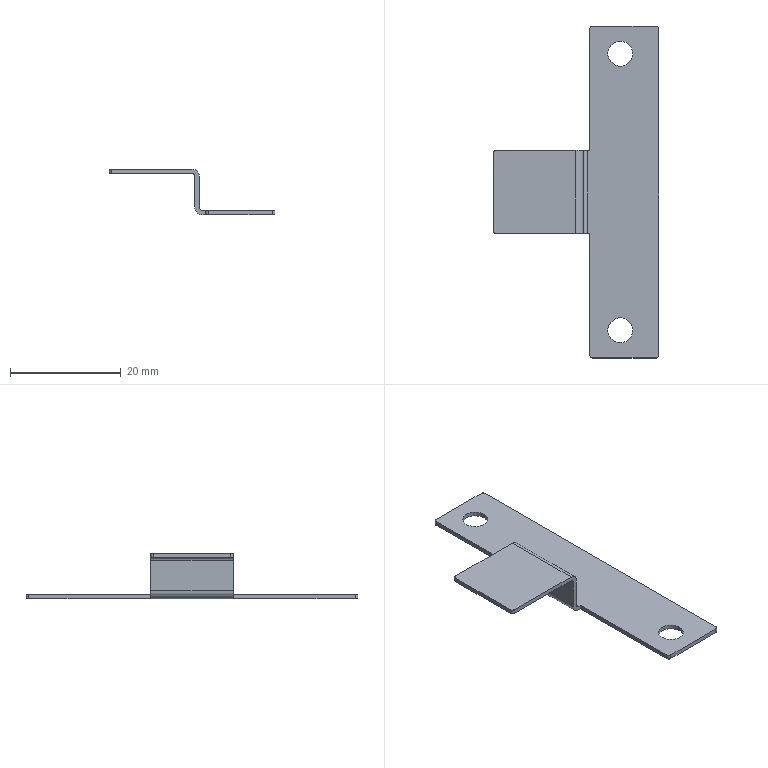Part | STEP file | 复件 FHB175-012^FHB175S-PRW-P40(马达RightUpper折-400W伺服电机) | 1 solid | 28 faces | box 30 x 60 x 8.3 mm | volume 863.995 mm3 | cylinder 14 | plane 14 | commonest cylinder face diameters 1 x7 4.5 x4 1.4 x1 2.6 x1 3 x1
STEP:
#1=CARTESIAN_POINT('',(7.253,-3.586,0.));
#2=VERTEX_POINT('',#1);
#3=CARTESIAN_POINT('',(11.753,-3.586,0.));
#4=VERTEX_POINT('',#3);
#5=CARTESIAN_POINT('',(9.503,-3.586,0.));
#6=DIRECTION('',(0.,0.,1.));
#7=DIRECTION('',(1.,0.,0.));
#8=AXIS2_PLACEMENT_3D('',#5,#6,#7);
#9=CIRCLE('',#8,2.25);
#10=EDGE_CURVE('',#2,#4,#9,.T.);
#11=ORIENTED_EDGE('',*,*,#10,.F.);
#12=CARTESIAN_POINT('',(7.253,-3.586,0.8));
#13=VERTEX_POINT('',#12);
#14=CARTESIAN_POINT('',(7.253,-3.586,0.8));
#15=DIRECTION('',(0.,0.,1.));
#16=VECTOR('',#15,1000.);
#17=LINE('',#14,#16);
#18=EDGE_CURVE('',#2,#13,#17,.T.);
#19=ORIENTED_EDGE('',*,*,#18,.T.);
#20=CARTESIAN_POINT('',(11.753,-3.586,0.8));
#21=VERTEX_POINT('',#20);
#22=CARTESIAN_POINT('',(9.503,-3.586,0.8));
#23=DIRECTION('',(0.,0.,-1.));
#24=DIRECTION('',(1.,0.,0.));
#25=AXIS2_PLACEMENT_3D('',#22,#23,#24);
#26=CIRCLE('',#25,2.25);
#27=EDGE_CURVE('',#21,#13,#26,.T.);
#28=ORIENTED_EDGE('',*,*,#27,.F.);
#29=CARTESIAN_POINT('',(11.753,-3.586,0.8));
#30=DIRECTION('',(0.,0.,1.));
#31=VECTOR('',#30,1000.);
#32=LINE('',#29,#31);
#33=EDGE_CURVE('',#4,#21,#32,.T.);
#34=ORIENTED_EDGE('',*,*,#33,.F.);
#35=EDGE_LOOP('',(#11,#19,#28,#34));
#36=FACE_OUTER_BOUND('',#35,.T.);
#37=CARTESIAN_POINT('',(9.503,-3.586,0.8));
#38=DIRECTION('',(0.,0.,1.));
#39=DIRECTION('',(1.,0.,0.));
#40=AXIS2_PLACEMENT_3D('',#37,#38,#39);
#41=CYLINDRICAL_SURFACE('',#40,2.25);
#42=ADVANCED_FACE('',(#36),#41,.F.);
#43=CARTESIAN_POINT('',(7.253,46.414,0.));
#44=VERTEX_POINT('',#43);
#45=CARTESIAN_POINT('',(11.753,46.414,0.));
#46=VERTEX_POINT('',#45);
#47=CARTESIAN_POINT('',(9.503,46.414,0.));
#48=DIRECTION('',(0.,0.,1.));
#49=DIRECTION('',(1.,0.,0.));
#50=AXIS2_PLACEMENT_3D('',#47,#48,#49);
#51=CIRCLE('',#50,2.25);
#52=EDGE_CURVE('',#44,#46,#51,.T.);
#53=ORIENTED_EDGE('',*,*,#52,.F.);
#54=CARTESIAN_POINT('',(7.253,46.414,0.8));
#55=VERTEX_POINT('',#54);
#56=CARTESIAN_POINT('',(7.253,46.414,0.8));
#57=DIRECTION('',(0.,0.,1.));
#58=VECTOR('',#57,1000.);
#59=LINE('',#56,#58);
#60=EDGE_CURVE('',#44,#55,#59,.T.);
#61=ORIENTED_EDGE('',*,*,#60,.T.);
#62=CARTESIAN_POINT('',(11.753,46.414,0.8));
#63=VERTEX_POINT('',#62);
#64=CARTESIAN_POINT('',(9.503,46.414,0.8));
#65=DIRECTION('',(0.,0.,-1.));
#66=DIRECTION('',(1.,0.,0.));
#67=AXIS2_PLACEMENT_3D('',#64,#65,#66);
#68=CIRCLE('',#67,2.25);
#69=EDGE_CURVE('',#63,#55,#68,.T.);
#70=ORIENTED_EDGE('',*,*,#69,.F.);
#71=CARTESIAN_POINT('',(11.753,46.414,0.8));
#72=DIRECTION('',(0.,0.,1.));
#73=VECTOR('',#72,1000.);
#74=LINE('',#71,#73);
#75=EDGE_CURVE('',#46,#63,#74,.T.);
#76=ORIENTED_EDGE('',*,*,#75,.F.);
#77=EDGE_LOOP('',(#53,#61,#70,#76));
#78=FACE_OUTER_BOUND('',#77,.T.);
#79=CARTESIAN_POINT('',(9.503,46.414,0.8));
#80=DIRECTION('',(0.,0.,1.));
#81=DIRECTION('',(1.,0.,0.));
#82=AXIS2_PLACEMENT_3D('',#79,#80,#81);
#83=CYLINDRICAL_SURFACE('',#82,2.25);
#84=ADVANCED_FACE('',(#78),#83,.F.);
#85=CARTESIAN_POINT('',(16.503,50.914,0.));
#86=VERTEX_POINT('',#85);
#87=CARTESIAN_POINT('',(16.503,-8.086,0.));
#88=VERTEX_POINT('',#87);
#89=CARTESIAN_POINT('',(16.503,0.,0.));
#90=DIRECTION('',(0.,-1.,0.));
#91=VECTOR('',#90,1000.);
#92=LINE('',#89,#91);
#93=EDGE_CURVE('',#86,#88,#92,.T.);
#94=ORIENTED_EDGE('',*,*,#93,.T.);
#95=CARTESIAN_POINT('',(16.003,-8.586,0.));
#96=VERTEX_POINT('',#95);
#97=CARTESIAN_POINT('',(16.003,-8.086,0.));
#98=DIRECTION('',(0.,0.,-1.));
#99=DIRECTION('',(-1.,0.,0.));
#100=AXIS2_PLACEMENT_3D('',#97,#98,#99);
#101=CIRCLE('',#100,0.5);
#102=EDGE_CURVE('',#88,#96,#101,.T.);
#103=ORIENTED_EDGE('',*,*,#102,.T.);
#104=CARTESIAN_POINT('',(4.503,-8.586,0.));
#105=VERTEX_POINT('',#104);
#106=CARTESIAN_POINT('',(0.,-8.586,0.));
#107=DIRECTION('',(-1.,0.,0.));
#108=VECTOR('',#107,1000.);
#109=LINE('',#106,#108);
#110=EDGE_CURVE('',#96,#105,#109,.T.);
#111=ORIENTED_EDGE('',*,*,#110,.T.);
#112=CARTESIAN_POINT('',(4.003,-8.086,0.));
#113=VERTEX_POINT('',#112);
#114=CARTESIAN_POINT('',(4.503,-8.086,0.));
#115=DIRECTION('',(0.,0.,-1.));
#116=DIRECTION('',(1.,0.,0.));
#117=AXIS2_PLACEMENT_3D('',#114,#115,#116);
#118=CIRCLE('',#117,0.5);
#119=EDGE_CURVE('',#105,#113,#118,.T.);
#120=ORIENTED_EDGE('',*,*,#119,.T.);
#121=CARTESIAN_POINT('',(4.003,13.914,0.));
#122=VERTEX_POINT('',#121);
#123=CARTESIAN_POINT('',(4.003,0.,0.));
#124=DIRECTION('',(0.,1.,0.));
#125=VECTOR('',#124,1000.);
#126=LINE('',#123,#125);
#127=EDGE_CURVE('',#113,#122,#126,.T.);
#128=ORIENTED_EDGE('',*,*,#127,.T.);
#129=CARTESIAN_POINT('',(3.503,13.914,0.));
#130=VERTEX_POINT('',#129);
#131=CARTESIAN_POINT('',(0.,13.914,0.));
#132=DIRECTION('',(-1.,0.,0.));
#133=VECTOR('',#132,1000.);
#134=LINE('',#131,#133);
#135=EDGE_CURVE('',#122,#130,#134,.T.);
#136=ORIENTED_EDGE('',*,*,#135,.T.);
#137=CARTESIAN_POINT('',(3.503,28.914,0.));
#138=VERTEX_POINT('',#137);
#139=CARTESIAN_POINT('',(3.503,0.,0.));
#140=DIRECTION('',(0.,1.,0.));
#141=VECTOR('',#140,1000.);
#142=LINE('',#139,#141);
#143=EDGE_CURVE('',#130,#138,#142,.T.);
#144=ORIENTED_EDGE('',*,*,#143,.T.);
#145=CARTESIAN_POINT('',(4.003,28.914,0.));
#146=VERTEX_POINT('',#145);
#147=CARTESIAN_POINT('',(0.,28.914,0.));
#148=DIRECTION('',(1.,0.,0.));
#149=VECTOR('',#148,1000.);
#150=LINE('',#147,#149);
#151=EDGE_CURVE('',#138,#146,#150,.T.);
#152=ORIENTED_EDGE('',*,*,#151,.T.);
#153=CARTESIAN_POINT('',(4.003,50.914,0.));
#154=VERTEX_POINT('',#153);
#155=CARTESIAN_POINT('',(4.003,0.,0.));
#156=DIRECTION('',(0.,1.,0.));
#157=VECTOR('',#156,1000.);
#158=LINE('',#155,#157);
#159=EDGE_CURVE('',#146,#154,#158,.T.);
#160=ORIENTED_EDGE('',*,*,#159,.T.);
#161=CARTESIAN_POINT('',(4.503,51.414,0.));
#162=VERTEX_POINT('',#161);
#163=CARTESIAN_POINT('',(4.503,50.914,0.));
#164=DIRECTION('',(0.,0.,-1.));
#165=DIRECTION('',(1.,0.,0.));
#166=AXIS2_PLACEMENT_3D('',#163,#164,#165);
#167=CIRCLE('',#166,0.5);
#168=EDGE_CURVE('',#154,#162,#167,.T.);
#169=ORIENTED_EDGE('',*,*,#168,.T.);
#170=CARTESIAN_POINT('',(16.003,51.414,0.));
#171=VERTEX_POINT('',#170);
#172=CARTESIAN_POINT('',(0.,51.414,0.));
#173=DIRECTION('',(1.,0.,0.));
#174=VECTOR('',#173,1000.);
#175=LINE('',#172,#174);
#176=EDGE_CURVE('',#162,#171,#175,.T.);
#177=ORIENTED_EDGE('',*,*,#176,.T.);
#178=CARTESIAN_POINT('',(16.003,50.914,0.));
#179=DIRECTION('',(0.,0.,-1.));
#180=DIRECTION('',(-1.,0.,0.));
#181=AXIS2_PLACEMENT_3D('',#178,#179,#180);
#182=CIRCLE('',#181,0.5);
#183=EDGE_CURVE('',#171,#86,#182,.T.);
#184=ORIENTED_EDGE('',*,*,#183,.T.);
#185=EDGE_LOOP('',(#94,#103,#111,#120,#128,#136,#144,#152,#160,#169,#177,#184));
#186=FACE_OUTER_BOUND('',#185,.T.);
#187=CARTESIAN_POINT('',(9.503,-3.586,0.));
#188=DIRECTION('',(0.,0.,1.));
#189=DIRECTION('',(1.,0.,0.));
#190=AXIS2_PLACEMENT_3D('',#187,#188,#189);
#191=CIRCLE('',#190,2.25);
#192=EDGE_CURVE('',#4,#2,#191,.T.);
#193=ORIENTED_EDGE('',*,*,#192,.T.);
#194=ORIENTED_EDGE('',*,*,#10,.T.);
#195=EDGE_LOOP('',(#193,#194));
#196=FACE_BOUND('',#195,.T.);
#197=CARTESIAN_POINT('',(9.503,46.414,0.));
#198=DIRECTION('',(0.,0.,1.));
#199=DIRECTION('',(1.,0.,0.));
#200=AXIS2_PLACEMENT_3D('',#197,#198,#199);
#201=CIRCLE('',#200,2.25);
#202=EDGE_CURVE('',#46,#44,#201,.T.);
#203=ORIENTED_EDGE('',*,*,#202,.T.);
#204=ORIENTED_EDGE('',*,*,#52,.T.);
#205=EDGE_LOOP('',(#203,#204));
#206=FACE_BOUND('',#205,.T.);
#207=CARTESIAN_POINT('',(0.,0.,0.));
#208=DIRECTION('',(0.,0.,-1.));
#209=DIRECTION('',(-1.,0.,0.));
#210=AXIS2_PLACEMENT_3D('',#207,#208,#209);
#211=PLANE('',#210);
#212=ADVANCED_FACE('',(#186,#196,#206),#211,.T.);
#213=ORIENTED_EDGE('',*,*,#102,.F.);
#214=CARTESIAN_POINT('',(16.503,-8.086,0.8));
#215=VERTEX_POINT('',#214);
#216=CARTESIAN_POINT('',(16.503,-8.086,0.8));
#217=DIRECTION('',(0.,0.,1.));
#218=VECTOR('',#217,1000.);
#219=LINE('',#216,#218);
#220=EDGE_CURVE('',#88,#215,#219,.T.);
#221=ORIENTED_EDGE('',*,*,#220,.T.);
#222=CARTESIAN_POINT('',(16.003,-8.586,0.8));
#223=VERTEX_POINT('',#222);
#224=CARTESIAN_POINT('',(16.003,-8.086,0.8));
#225=DIRECTION('',(0.,0.,-1.));
#226=DIRECTION('',(-1.,0.,0.));
#227=AXIS2_PLACEMENT_3D('',#224,#225,#226);
#228=CIRCLE('',#227,0.5);
#229=EDGE_CURVE('',#215,#223,#228,.T.);
#230=ORIENTED_EDGE('',*,*,#229,.T.);
#231=CARTESIAN_POINT('',(16.003,-8.586,0.8));
#232=DIRECTION('',(0.,0.,-1.));
#233=VECTOR('',#232,1000.);
#234=LINE('',#231,#233);
#235=EDGE_CURVE('',#223,#96,#234,.T.);
#236=ORIENTED_EDGE('',*,*,#235,.T.);
#237=EDGE_LOOP('',(#213,#221,#230,#236));
#238=FACE_OUTER_BOUND('',#237,.T.);
#239=CARTESIAN_POINT('',(16.003,-8.086,0.8));
#240=DIRECTION('',(0.,0.,-1.));
#241=DIRECTION('',(-1.,0.,0.));
#242=AXIS2_PLACEMENT_3D('',#239,#240,#241);
#243=CYLINDRICAL_SURFACE('',#242,0.5);
#244=ADVANCED_FACE('',(#238),#243,.T.);
#245=ORIENTED_EDGE('',*,*,#220,.F.);
#246=ORIENTED_EDGE('',*,*,#93,.F.);
#247=CARTESIAN_POINT('',(16.503,50.914,0.8));
#248=VERTEX_POINT('',#247);
#249=CARTESIAN_POINT('',(16.503,50.914,0.8));
#250=DIRECTION('',(0.,0.,-1.));
#251=VECTOR('',#250,1000.);
#252=LINE('',#249,#251);
#253=EDGE_CURVE('',#248,#86,#252,.T.);
#254=ORIENTED_EDGE('',*,*,#253,.F.);
#255=CARTESIAN_POINT('',(16.503,51.414,0.8));
#256=DIRECTION('',(0.,1.,0.));
#257=VECTOR('',#256,1000.);
#258=LINE('',#255,#257);
#259=EDGE_CURVE('',#215,#248,#258,.T.);
#260=ORIENTED_EDGE('',*,*,#259,.F.);
#261=EDGE_LOOP('',(#245,#246,#254,#260));
#262=FACE_OUTER_BOUND('',#261,.T.);
#263=CARTESIAN_POINT('',(16.503,51.414,0.8));
#264=DIRECTION('',(-1.,0.,0.));
#265=DIRECTION('',(0.,-1.,0.));
#266=AXIS2_PLACEMENT_3D('',#263,#264,#265);
#267=PLANE('',#266);
#268=ADVANCED_FACE('',(#262),#267,.F.);
#269=ORIENTED_EDGE('',*,*,#183,.F.);
#270=CARTESIAN_POINT('',(16.003,51.414,0.8));
#271=VERTEX_POINT('',#270);
#272=CARTESIAN_POINT('',(16.003,51.414,0.8));
#273=DIRECTION('',(0.,0.,1.));
#274=VECTOR('',#273,1000.);
#275=LINE('',#272,#274);
#276=EDGE_CURVE('',#171,#271,#275,.T.);
#277=ORIENTED_EDGE('',*,*,#276,.T.);
#278=CARTESIAN_POINT('',(16.003,50.914,0.8));
#279=DIRECTION('',(0.,0.,-1.));
#280=DIRECTION('',(-1.,0.,0.));
#281=AXIS2_PLACEMENT_3D('',#278,#279,#280);
#282=CIRCLE('',#281,0.5);
#283=EDGE_CURVE('',#271,#248,#282,.T.);
#284=ORIENTED_EDGE('',*,*,#283,.T.);
#285=ORIENTED_EDGE('',*,*,#253,.T.);
#286=EDGE_LOOP('',(#269,#277,#284,#285));
#287=FACE_OUTER_BOUND('',#286,.T.);
#288=CARTESIAN_POINT('',(16.003,50.914,0.8));
#289=DIRECTION('',(0.,0.,-1.));
#290=DIRECTION('',(-1.,0.,0.));
#291=AXIS2_PLACEMENT_3D('',#288,#289,#290);
#292=CYLINDRICAL_SURFACE('',#291,0.5);
#293=ADVANCED_FACE('',(#287),#292,.T.);
#294=CARTESIAN_POINT('',(4.503,51.414,0.8));
#295=VERTEX_POINT('',#294);
#296=CARTESIAN_POINT('',(4.503,51.414,0.8));
#297=DIRECTION('',(0.,0.,-1.));
#298=VECTOR('',#297,1000.);
#299=LINE('',#296,#298);
#300=EDGE_CURVE('',#295,#162,#299,.T.);
#301=ORIENTED_EDGE('',*,*,#300,.F.);
#302=CARTESIAN_POINT('',(16.503,51.414,0.8));
#303=DIRECTION('',(-1.,0.,0.));
#304=VECTOR('',#303,1000.);
#305=LINE('',#302,#304);
#306=EDGE_CURVE('',#271,#295,#305,.T.);
#307=ORIENTED_EDGE('',*,*,#306,.F.);
#308=ORIENTED_EDGE('',*,*,#276,.F.);
#309=ORIENTED_EDGE('',*,*,#176,.F.);
#310=EDGE_LOOP('',(#301,#307,#308,#309));
#311=FACE_OUTER_BOUND('',#310,.T.);
#312=CARTESIAN_POINT('',(16.503,51.414,0.8));
#313=DIRECTION('',(0.,-1.,0.));
#314=DIRECTION('',(0.,0.,-1.));
#315=AXIS2_PLACEMENT_3D('',#312,#313,#314);
#316=PLANE('',#315);
#317=ADVANCED_FACE('',(#311),#316,.F.);
#318=CARTESIAN_POINT('',(4.003,50.914,0.8));
#319=VERTEX_POINT('',#318);
#320=CARTESIAN_POINT('',(4.503,50.914,0.8));
#321=DIRECTION('',(0.,0.,-1.));
#322=DIRECTION('',(1.,0.,0.));
#323=AXIS2_PLACEMENT_3D('',#320,#321,#322);
#324=CIRCLE('',#323,0.5);
#325=EDGE_CURVE('',#319,#295,#324,.T.);
#326=ORIENTED_EDGE('',*,*,#325,.T.);
#327=ORIENTED_EDGE('',*,*,#300,.T.);
#328=ORIENTED_EDGE('',*,*,#168,.F.);
#329=CARTESIAN_POINT('',(4.003,50.914,0.8));
#330=DIRECTION('',(0.,0.,1.));
#331=VECTOR('',#330,1000.);
#332=LINE('',#329,#331);
#333=EDGE_CURVE('',#154,#319,#332,.T.);
#334=ORIENTED_EDGE('',*,*,#333,.T.);
#335=EDGE_LOOP('',(#326,#327,#328,#334));
#336=FACE_OUTER_BOUND('',#335,.T.);
#337=CARTESIAN_POINT('',(4.503,50.914,0.8));
#338=DIRECTION('',(0.,0.,1.));
#339=DIRECTION('',(1.,0.,0.));
#340=AXIS2_PLACEMENT_3D('',#337,#338,#339);
#341=CYLINDRICAL_SURFACE('',#340,0.5);
#342=ADVANCED_FACE('',(#336),#341,.T.);
#343=ORIENTED_EDGE('',*,*,#333,.F.);
#344=ORIENTED_EDGE('',*,*,#159,.F.);
#345=CARTESIAN_POINT('',(4.003,28.914,0.8));
#346=VERTEX_POINT('',#345);
#347=CARTESIAN_POINT('',(4.003,28.914,0.));
#348=DIRECTION('',(0.,0.,-1.));
#349=VECTOR('',#348,1000.);
#350=LINE('',#347,#349);
#351=EDGE_CURVE('',#346,#146,#350,.T.);
#352=ORIENTED_EDGE('',*,*,#351,.F.);
#353=CARTESIAN_POINT('',(4.003,51.414,0.8));
#354=DIRECTION('',(0.,-1.,0.));
#355=VECTOR('',#354,1000.);
#356=LINE('',#353,#355);
#357=EDGE_CURVE('',#319,#346,#356,.T.);
#358=ORIENTED_EDGE('',*,*,#357,.F.);
#359=EDGE_LOOP('',(#343,#344,#352,#358));
#360=FACE_OUTER_BOUND('',#359,.T.);
#361=CARTESIAN_POINT('',(4.003,51.414,0.));
#362=DIRECTION('',(1.,0.,0.));
#363=DIRECTION('',(0.,1.,0.));
#364=AXIS2_PLACEMENT_3D('',#361,#362,#363);
#365=PLANE('',#364);
#366=ADVANCED_FACE('',(#360),#365,.F.);
#367=ORIENTED_EDGE('',*,*,#351,.T.);
#368=ORIENTED_EDGE('',*,*,#151,.F.);
#369=CARTESIAN_POINT('',(2.003,28.914,1.5));
#370=VERTEX_POINT('',#369);
#371=CARTESIAN_POINT('',(3.503,28.914,1.5));
#372=DIRECTION('',(0.,-1.,0.));
#373=DIRECTION('',(0.,0.,-1.));
#374=AXIS2_PLACEMENT_3D('',#371,#372,#373);
#375=CIRCLE('',#374,1.5);
#376=EDGE_CURVE('',#370,#138,#375,.T.);
#377=ORIENTED_EDGE('',*,*,#376,.F.);
#378=CARTESIAN_POINT('',(2.003,28.914,7.));
#379=VERTEX_POINT('',#378);
#380=CARTESIAN_POINT('',(2.003,28.914,0.));
#381=DIRECTION('',(0.,0.,1.));
#382=VECTOR('',#381,1000.);
#383=LINE('',#380,#382);
#384=EDGE_CURVE('',#370,#379,#383,.T.);
#385=ORIENTED_EDGE('',*,*,#384,.T.);
#386=CARTESIAN_POINT('',(1.503,28.914,7.5));
#387=VERTEX_POINT('',#386);
#388=CARTESIAN_POINT('',(1.503,28.914,7.));
#389=DIRECTION('',(0.,1.,0.));
#390=DIRECTION('',(0.,0.,1.));
#391=AXIS2_PLACEMENT_3D('',#388,#389,#390);
#392=CIRCLE('',#391,0.5);
#393=EDGE_CURVE('',#387,#379,#392,.T.);
#394=ORIENTED_EDGE('',*,*,#393,.F.);
#395=CARTESIAN_POINT('',(-12.997,28.914,7.5));
#396=VERTEX_POINT('',#395);
#397=CARTESIAN_POINT('',(0.,28.914,7.5));
#398=DIRECTION('',(-1.,0.,0.));
#399=VECTOR('',#398,1000.);
#400=LINE('',#397,#399);
#401=EDGE_CURVE('',#387,#396,#400,.T.);
#402=ORIENTED_EDGE('',*,*,#401,.T.);
#403=CARTESIAN_POINT('',(-12.997,28.914,8.3));
#404=VERTEX_POINT('',#403);
#405=CARTESIAN_POINT('',(-12.997,28.914,8.3));
#406=DIRECTION('',(0.,0.,-1.));
#407=VECTOR('',#406,1000.);
#408=LINE('',#405,#407);
#409=EDGE_CURVE('',#404,#396,#408,.T.);
#410=ORIENTED_EDGE('',*,*,#409,.F.);
#411=CARTESIAN_POINT('',(1.503,28.914,8.3));
#412=VERTEX_POINT('',#411);
#413=CARTESIAN_POINT('',(2.003,28.914,8.3));
#414=DIRECTION('',(1.,0.,0.));
#415=VECTOR('',#414,1000.);
#416=LINE('',#413,#415);
#417=EDGE_CURVE('',#404,#412,#416,.T.);
#418=ORIENTED_EDGE('',*,*,#417,.T.);
#419=CARTESIAN_POINT('',(2.803,28.914,7.));
#420=VERTEX_POINT('',#419);
#421=CARTESIAN_POINT('',(1.503,28.914,7.));
#422=DIRECTION('',(0.,-1.,0.));
#423=DIRECTION('',(0.,0.,1.));
#424=AXIS2_PLACEMENT_3D('',#421,#422,#423);
#425=CIRCLE('',#424,1.3);
#426=EDGE_CURVE('',#420,#412,#425,.T.);
#427=ORIENTED_EDGE('',*,*,#426,.F.);
#428=CARTESIAN_POINT('',(2.803,28.914,1.5));
#429=VERTEX_POINT('',#428);
#430=CARTESIAN_POINT('',(2.803,28.914,0.8));
#431=DIRECTION('',(0.,0.,1.));
#432=VECTOR('',#431,1000.);
#433=LINE('',#430,#432);
#434=EDGE_CURVE('',#429,#420,#433,.T.);
#435=ORIENTED_EDGE('',*,*,#434,.F.);
#436=CARTESIAN_POINT('',(3.503,28.914,0.8));
#437=VERTEX_POINT('',#436);
#438=CARTESIAN_POINT('',(3.503,28.914,1.5));
#439=DIRECTION('',(0.,-1.,0.));
#440=DIRECTION('',(0.,0.,-1.));
#441=AXIS2_PLACEMENT_3D('',#438,#439,#440);
#442=CIRCLE('',#441,0.7);
#443=EDGE_CURVE('',#429,#437,#442,.T.);
#444=ORIENTED_EDGE('',*,*,#443,.T.);
#445=CARTESIAN_POINT('',(4.003,28.914,0.8));
#446=DIRECTION('',(-1.,0.,0.));
#447=VECTOR('',#446,1000.);
#448=LINE('',#445,#447);
#449=EDGE_CURVE('',#346,#437,#448,.T.);
#450=ORIENTED_EDGE('',*,*,#449,.F.);
#451=EDGE_LOOP('',(#367,#368,#377,#385,#394,#402,#410,#418,#427,#435,#444,#450));
#452=FACE_OUTER_BOUND('',#451,.T.);
#453=CARTESIAN_POINT('',(4.003,28.914,0.));
#454=DIRECTION('',(0.,-1.,0.));
#455=DIRECTION('',(0.,0.,-1.));
#456=AXIS2_PLACEMENT_3D('',#453,#454,#455);
#457=PLANE('',#456);
#458=ADVANCED_FACE('',(#452),#457,.F.);
#459=CARTESIAN_POINT('',(2.003,13.914,1.5));
#460=VERTEX_POINT('',#459);
#461=CARTESIAN_POINT('',(2.003,13.914,1.5));
#462=DIRECTION('',(0.,1.,0.));
#463=VECTOR('',#462,1000.);
#464=LINE('',#461,#463);
#465=EDGE_CURVE('',#460,#370,#464,.T.);
#466=ORIENTED_EDGE('',*,*,#465,.T.);
#467=ORIENTED_EDGE('',*,*,#376,.T.);
#468=ORIENTED_EDGE('',*,*,#143,.F.);
#469=CARTESIAN_POINT('',(3.503,13.914,1.5));
#470=DIRECTION('',(0.,1.,0.));
#471=DIRECTION('',(0.,0.,-1.));
#472=AXIS2_PLACEMENT_3D('',#469,#470,#471);
#473=CIRCLE('',#472,1.5);
#474=EDGE_CURVE('',#130,#460,#473,.T.);
#475=ORIENTED_EDGE('',*,*,#474,.T.);
#476=EDGE_LOOP('',(#466,#467,#468,#475));
#477=FACE_OUTER_BOUND('',#476,.T.);
#478=CARTESIAN_POINT('',(3.503,13.914,1.5));
#479=DIRECTION('',(0.,-1.,0.));
#480=DIRECTION('',(0.,0.,-1.));
#481=AXIS2_PLACEMENT_3D('',#478,#479,#480);
#482=CYLINDRICAL_SURFACE('',#481,1.5);
#483=ADVANCED_FACE('',(#477),#482,.T.);
#484=CARTESIAN_POINT('',(4.003,13.914,0.8));
#485=VERTEX_POINT('',#484);
#486=CARTESIAN_POINT('',(4.003,13.914,0.));
#487=DIRECTION('',(0.,0.,-1.));
#488=VECTOR('',#487,1000.);
#489=LINE('',#486,#488);
#490=EDGE_CURVE('',#485,#122,#489,.T.);
#491=ORIENTED_EDGE('',*,*,#490,.F.);
#492=CARTESIAN_POINT('',(3.503,13.914,0.8));
#493=VERTEX_POINT('',#492);
#494=CARTESIAN_POINT('',(4.003,13.914,0.8));
#495=DIRECTION('',(1.,0.,0.));
#496=VECTOR('',#495,1000.);
#497=LINE('',#494,#496);
#498=EDGE_CURVE('',#493,#485,#497,.T.);
#499=ORIENTED_EDGE('',*,*,#498,.F.);
#500=CARTESIAN_POINT('',(2.803,13.914,1.5));
#501=VERTEX_POINT('',#500);
#502=CARTESIAN_POINT('',(3.503,13.914,1.5));
#503=DIRECTION('',(0.,-1.,0.));
#504=DIRECTION('',(0.,0.,-1.));
#505=AXIS2_PLACEMENT_3D('',#502,#503,#504);
#506=CIRCLE('',#505,0.7);
#507=EDGE_CURVE('',#501,#493,#506,.T.);
#508=ORIENTED_EDGE('',*,*,#507,.F.);
#509=CARTESIAN_POINT('',(2.803,13.914,7.));
#510=VERTEX_POINT('',#509);
#511=CARTESIAN_POINT('',(2.803,13.914,8.3));
#512=DIRECTION('',(0.,0.,-1.));
#513=VECTOR('',#512,1000.);
#514=LINE('',#511,#513);
#515=EDGE_CURVE('',#510,#501,#514,.T.);
#516=ORIENTED_EDGE('',*,*,#515,.F.);
#517=CARTESIAN_POINT('',(1.503,13.914,8.3));
#518=VERTEX_POINT('',#517);
#519=CARTESIAN_POINT('',(1.503,13.914,7.));
#520=DIRECTION('',(0.,1.,0.));
#521=DIRECTION('',(0.,0.,1.));
#522=AXIS2_PLACEMENT_3D('',#519,#520,#521);
#523=CIRCLE('',#522,1.3);
#524=EDGE_CURVE('',#518,#510,#523,.T.);
#525=ORIENTED_EDGE('',*,*,#524,.F.);
#526=CARTESIAN_POINT('',(-12.997,13.914,8.3));
#527=VERTEX_POINT('',#526);
#528=CARTESIAN_POINT('',(-13.497,13.914,8.3));
#529=DIRECTION('',(-1.,0.,0.));
#530=VECTOR('',#529,1000.);
#531=LINE('',#528,#530);
#532=EDGE_CURVE('',#518,#527,#531,.T.);
#533=ORIENTED_EDGE('',*,*,#532,.T.);
#534=CARTESIAN_POINT('',(-12.997,13.914,7.5));
#535=VERTEX_POINT('',#534);
#536=CARTESIAN_POINT('',(-12.997,13.914,8.3));
#537=DIRECTION('',(0.,0.,-1.));
#538=VECTOR('',#537,1000.);
#539=LINE('',#536,#538);
#540=EDGE_CURVE('',#527,#535,#539,.T.);
#541=ORIENTED_EDGE('',*,*,#540,.T.);
#542=CARTESIAN_POINT('',(1.503,13.914,7.5));
#543=VERTEX_POINT('',#542);
#544=CARTESIAN_POINT('',(0.,13.914,7.5));
#545=DIRECTION('',(1.,0.,0.));
#546=VECTOR('',#545,1000.);
#547=LINE('',#544,#546);
#548=EDGE_CURVE('',#535,#543,#547,.T.);
#549=ORIENTED_EDGE('',*,*,#548,.T.);
#550=CARTESIAN_POINT('',(2.003,13.914,7.));
#551=VERTEX_POINT('',#550);
#552=CARTESIAN_POINT('',(1.503,13.914,7.));
#553=DIRECTION('',(0.,1.,0.));
#554=DIRECTION('',(0.,0.,1.));
#555=AXIS2_PLACEMENT_3D('',#552,#553,#554);
#556=CIRCLE('',#555,0.5);
#557=EDGE_CURVE('',#543,#551,#556,.T.);
#558=ORIENTED_EDGE('',*,*,#557,.T.);
#559=CARTESIAN_POINT('',(2.003,13.914,0.));
#560=DIRECTION('',(0.,0.,-1.));
#561=VECTOR('',#560,1000.);
#562=LINE('',#559,#561);
#563=EDGE_CURVE('',#551,#460,#562,.T.);
#564=ORIENTED_EDGE('',*,*,#563,.T.);
#565=ORIENTED_EDGE('',*,*,#474,.F.);
#566=ORIENTED_EDGE('',*,*,#135,.F.);
#567=EDGE_LOOP('',(#491,#499,#508,#516,#525,#533,#541,#549,#558,#564,#565,#566));
#568=FACE_OUTER_BOUND('',#567,.T.);
#569=CARTESIAN_POINT('',(4.003,13.914,0.));
#570=DIRECTION('',(0.,1.,0.));
#571=DIRECTION('',(0.,0.,1.));
#572=AXIS2_PLACEMENT_3D('',#569,#570,#571);
#573=PLANE('',#572);
#574=ADVANCED_FACE('',(#568),#573,.F.);
#575=CARTESIAN_POINT('',(4.003,-8.086,0.8));
#576=VERTEX_POINT('',#575);
#577=CARTESIAN_POINT('',(4.003,-8.086,0.));
#578=DIRECTION('',(0.,0.,-1.));
#579=VECTOR('',#578,1000.);
#580=LINE('',#577,#579);
#581=EDGE_CURVE('',#576,#113,#580,.T.);
#582=ORIENTED_EDGE('',*,*,#581,.F.);
#583=CARTESIAN_POINT('',(4.003,-8.586,0.8));
#584=DIRECTION('',(0.,-1.,0.));
#585=VECTOR('',#584,1000.);
#586=LINE('',#583,#585);
#587=EDGE_CURVE('',#485,#576,#586,.T.);
#588=ORIENTED_EDGE('',*,*,#587,.F.);
#589=ORIENTED_EDGE('',*,*,#490,.T.);
#590=ORIENTED_EDGE('',*,*,#127,.F.);
#591=EDGE_LOOP('',(#582,#588,#589,#590));
#592=FACE_OUTER_BOUND('',#591,.T.);
#593=CARTESIAN_POINT('',(4.003,-8.586,0.));
#594=DIRECTION('',(1.,0.,0.));
#595=DIRECTION('',(0.,0.,-1.));
#596=AXIS2_PLACEMENT_3D('',#593,#594,#595);
#597=PLANE('',#596);
#598=ADVANCED_FACE('',(#592),#597,.F.);
#599=CARTESIAN_POINT('',(4.503,-8.586,0.8));
#600=VERTEX_POINT('',#599);
#601=CARTESIAN_POINT('',(4.503,-8.086,0.8));
#602=DIRECTION('',(0.,0.,-1.));
#603=DIRECTION('',(1.,0.,0.));
#604=AXIS2_PLACEMENT_3D('',#601,#602,#603);
#605=CIRCLE('',#604,0.5);
#606=EDGE_CURVE('',#600,#576,#605,.T.);
#607=ORIENTED_EDGE('',*,*,#606,.T.);
#608=ORIENTED_EDGE('',*,*,#581,.T.);
#609=ORIENTED_EDGE('',*,*,#119,.F.);
#610=CARTESIAN_POINT('',(4.503,-8.586,0.));
#611=DIRECTION('',(0.,0.,1.));
#612=VECTOR('',#611,1000.);
#613=LINE('',#610,#612);
#614=EDGE_CURVE('',#105,#600,#613,.T.);
#615=ORIENTED_EDGE('',*,*,#614,.T.);
#616=EDGE_LOOP('',(#607,#608,#609,#615));
#617=FACE_OUTER_BOUND('',#616,.T.);
#618=CARTESIAN_POINT('',(4.503,-8.086,0.));
#619=DIRECTION('',(0.,0.,1.));
#620=DIRECTION('',(1.,0.,0.));
#621=AXIS2_PLACEMENT_3D('',#618,#619,#620);
#622=CYLINDRICAL_SURFACE('',#621,0.5);
#623=ADVANCED_FACE('',(#617),#622,.T.);
#624=ORIENTED_EDGE('',*,*,#614,.F.);
#625=ORIENTED_EDGE('',*,*,#110,.F.);
#626=ORIENTED_EDGE('',*,*,#235,.F.);
#627=CARTESIAN_POINT('',(16.503,-8.586,0.8));
#628=DIRECTION('',(1.,0.,0.));
#629=VECTOR('',#628,1000.);
#630=LINE('',#627,#629);
#631=EDGE_CURVE('',#600,#223,#630,.T.);
#632=ORIENTED_EDGE('',*,*,#631,.F.);
#633=EDGE_LOOP('',(#624,#625,#626,#632));
#634=FACE_OUTER_BOUND('',#633,.T.);
#635=CARTESIAN_POINT('',(16.503,-8.586,0.8));
#636=DIRECTION('',(0.,1.,0.));
#637=DIRECTION('',(-1.,0.,0.));
#638=AXIS2_PLACEMENT_3D('',#635,#636,#637);
#639=PLANE('',#638);
#640=ADVANCED_FACE('',(#634),#639,.F.);
#641=ORIENTED_EDGE('',*,*,#18,.F.);
#642=ORIENTED_EDGE('',*,*,#192,.F.);
#643=ORIENTED_EDGE('',*,*,#33,.T.);
#644=CARTESIAN_POINT('',(9.503,-3.586,0.8));
#645=DIRECTION('',(0.,0.,-1.));
#646=DIRECTION('',(1.,0.,0.));
#647=AXIS2_PLACEMENT_3D('',#644,#645,#646);
#648=CIRCLE('',#647,2.25);
#649=EDGE_CURVE('',#13,#21,#648,.T.);
#650=ORIENTED_EDGE('',*,*,#649,.F.);
#651=EDGE_LOOP('',(#641,#642,#643,#650));
#652=FACE_OUTER_BOUND('',#651,.T.);
#653=CARTESIAN_POINT('',(9.503,-3.586,0.8));
#654=DIRECTION('',(0.,0.,1.));
#655=DIRECTION('',(1.,0.,0.));
#656=AXIS2_PLACEMENT_3D('',#653,#654,#655);
#657=CYLINDRICAL_SURFACE('',#656,2.25);
#658=ADVANCED_FACE('',(#652),#657,.F.);
#659=ORIENTED_EDGE('',*,*,#60,.F.);
#660=ORIENTED_EDGE('',*,*,#202,.F.);
#661=ORIENTED_EDGE('',*,*,#75,.T.);
#662=CARTESIAN_POINT('',(9.503,46.414,0.8));
#663=DIRECTION('',(0.,0.,-1.));
#664=DIRECTION('',(1.,0.,0.));
#665=AXIS2_PLACEMENT_3D('',#662,#663,#664);
#666=CIRCLE('',#665,2.25);
#667=EDGE_CURVE('',#55,#63,#666,.T.);
#668=ORIENTED_EDGE('',*,*,#667,.F.);
#669=EDGE_LOOP('',(#659,#660,#661,#668));
#670=FACE_OUTER_BOUND('',#669,.T.);
#671=CARTESIAN_POINT('',(9.503,46.414,0.8));
#672=DIRECTION('',(0.,0.,1.));
#673=DIRECTION('',(1.,0.,0.));
#674=AXIS2_PLACEMENT_3D('',#671,#672,#673);
#675=CYLINDRICAL_SURFACE('',#674,2.25);
#676=ADVANCED_FACE('',(#670),#675,.F.);
#677=ORIENTED_EDGE('',*,*,#606,.F.);
#678=ORIENTED_EDGE('',*,*,#631,.T.);
#679=ORIENTED_EDGE('',*,*,#229,.F.);
#680=ORIENTED_EDGE('',*,*,#259,.T.);
#681=ORIENTED_EDGE('',*,*,#283,.F.);
#682=ORIENTED_EDGE('',*,*,#306,.T.);
#683=ORIENTED_EDGE('',*,*,#325,.F.);
#684=ORIENTED_EDGE('',*,*,#357,.T.);
#685=ORIENTED_EDGE('',*,*,#449,.T.);
#686=CARTESIAN_POINT('',(3.503,0.,0.8));
#687=DIRECTION('',(0.,1.,0.));
#688=VECTOR('',#687,1000.);
#689=LINE('',#686,#688);
#690=EDGE_CURVE('',#493,#437,#689,.T.);
#691=ORIENTED_EDGE('',*,*,#690,.F.);
#692=ORIENTED_EDGE('',*,*,#498,.T.);
#693=ORIENTED_EDGE('',*,*,#587,.T.);
#694=EDGE_LOOP('',(#677,#678,#679,#680,#681,#682,#683,#684,#685,#691,#692,#693));
#695=FACE_OUTER_BOUND('',#694,.T.);
#696=ORIENTED_EDGE('',*,*,#27,.T.);
#697=ORIENTED_EDGE('',*,*,#649,.T.);
#698=EDGE_LOOP('',(#696,#697));
#699=FACE_BOUND('',#698,.T.);
#700=ORIENTED_EDGE('',*,*,#69,.T.);
#701=ORIENTED_EDGE('',*,*,#667,.T.);
#702=EDGE_LOOP('',(#700,#701));
#703=FACE_BOUND('',#702,.T.);
#704=CARTESIAN_POINT('',(0.,0.,0.8));
#705=DIRECTION('',(0.,0.,-1.));
#706=DIRECTION('',(-1.,0.,0.));
#707=AXIS2_PLACEMENT_3D('',#704,#705,#706);
#708=PLANE('',#707);
#709=ADVANCED_FACE('',(#695,#699,#703),#708,.F.);
#710=ORIENTED_EDGE('',*,*,#384,.F.);
#711=ORIENTED_EDGE('',*,*,#465,.F.);
#712=ORIENTED_EDGE('',*,*,#563,.F.);
#713=CARTESIAN_POINT('',(2.003,0.,7.));
#714=DIRECTION('',(0.,-1.,0.));
#715=VECTOR('',#714,1000.);
#716=LINE('',#713,#715);
#717=EDGE_CURVE('',#379,#551,#716,.T.);
#718=ORIENTED_EDGE('',*,*,#717,.F.);
#719=EDGE_LOOP('',(#710,#711,#712,#718));
#720=FACE_OUTER_BOUND('',#719,.T.);
#721=CARTESIAN_POINT('',(2.003,0.,0.));
#722=DIRECTION('',(1.,0.,0.));
#723=DIRECTION('',(0.,0.,-1.));
#724=AXIS2_PLACEMENT_3D('',#721,#722,#723);
#725=PLANE('',#724);
#726=ADVANCED_FACE('',(#720),#725,.F.);
#727=ORIENTED_EDGE('',*,*,#443,.F.);
#728=CARTESIAN_POINT('',(2.803,13.914,1.5));
#729=DIRECTION('',(0.,1.,0.));
#730=VECTOR('',#729,1000.);
#731=LINE('',#728,#730);
#732=EDGE_CURVE('',#501,#429,#731,.T.);
#733=ORIENTED_EDGE('',*,*,#732,.F.);
#734=ORIENTED_EDGE('',*,*,#507,.T.);
#735=ORIENTED_EDGE('',*,*,#690,.T.);
#736=EDGE_LOOP('',(#727,#733,#734,#735));
#737=FACE_OUTER_BOUND('',#736,.T.);
#738=CARTESIAN_POINT('',(3.503,13.914,1.5));
#739=DIRECTION('',(0.,-1.,0.));
#740=DIRECTION('',(0.,0.,-1.));
#741=AXIS2_PLACEMENT_3D('',#738,#739,#740);
#742=CYLINDRICAL_SURFACE('',#741,0.7);
#743=ADVANCED_FACE('',(#737),#742,.F.);
#744=ORIENTED_EDGE('',*,*,#557,.F.);
#745=CARTESIAN_POINT('',(1.503,28.914,7.5));
#746=DIRECTION('',(0.,-1.,0.));
#747=VECTOR('',#746,1000.);
#748=LINE('',#745,#747);
#749=EDGE_CURVE('',#387,#543,#748,.T.);
#750=ORIENTED_EDGE('',*,*,#749,.F.);
#751=ORIENTED_EDGE('',*,*,#393,.T.);
#752=ORIENTED_EDGE('',*,*,#717,.T.);
#753=EDGE_LOOP('',(#744,#750,#751,#752));
#754=FACE_OUTER_BOUND('',#753,.T.);
#755=CARTESIAN_POINT('',(1.503,28.914,7.));
#756=DIRECTION('',(0.,1.,0.));
#757=DIRECTION('',(0.,0.,1.));
#758=AXIS2_PLACEMENT_3D('',#755,#756,#757);
#759=CYLINDRICAL_SURFACE('',#758,0.5);
#760=ADVANCED_FACE('',(#754),#759,.F.);
#761=ORIENTED_EDGE('',*,*,#515,.T.);
#762=ORIENTED_EDGE('',*,*,#732,.T.);
#763=ORIENTED_EDGE('',*,*,#434,.T.);
#764=CARTESIAN_POINT('',(2.803,0.,7.));
#765=DIRECTION('',(0.,-1.,0.));
#766=VECTOR('',#765,1000.);
#767=LINE('',#764,#766);
#768=EDGE_CURVE('',#420,#510,#767,.T.);
#769=ORIENTED_EDGE('',*,*,#768,.T.);
#770=EDGE_LOOP('',(#761,#762,#763,#769));
#771=FACE_OUTER_BOUND('',#770,.T.);
#772=CARTESIAN_POINT('',(2.803,0.,0.));
#773=DIRECTION('',(1.,0.,0.));
#774=DIRECTION('',(0.,0.,-1.));
#775=AXIS2_PLACEMENT_3D('',#772,#773,#774);
#776=PLANE('',#775);
#777=ADVANCED_FACE('',(#771),#776,.T.);
#778=CARTESIAN_POINT('',(-13.497,28.414,7.5));
#779=VERTEX_POINT('',#778);
#780=CARTESIAN_POINT('',(-12.997,28.414,7.5));
#781=DIRECTION('',(0.,0.,1.));
#782=DIRECTION('',(-1.,0.,0.));
#783=AXIS2_PLACEMENT_3D('',#780,#781,#782);
#784=CIRCLE('',#783,0.5);
#785=EDGE_CURVE('',#396,#779,#784,.T.);
#786=ORIENTED_EDGE('',*,*,#785,.F.);
#787=ORIENTED_EDGE('',*,*,#401,.F.);
#788=ORIENTED_EDGE('',*,*,#749,.T.);
#789=ORIENTED_EDGE('',*,*,#548,.F.);
#790=CARTESIAN_POINT('',(-13.497,14.414,7.5));
#791=VERTEX_POINT('',#790);
#792=CARTESIAN_POINT('',(-12.997,14.414,7.5));
#793=DIRECTION('',(0.,0.,1.));
#794=DIRECTION('',(-1.,0.,0.));
#795=AXIS2_PLACEMENT_3D('',#792,#793,#794);
#796=CIRCLE('',#795,0.5);
#797=EDGE_CURVE('',#791,#535,#796,.T.);
#798=ORIENTED_EDGE('',*,*,#797,.F.);
#799=CARTESIAN_POINT('',(-13.497,0.,7.5));
#800=DIRECTION('',(0.,-1.,0.));
#801=VECTOR('',#800,1000.);
#802=LINE('',#799,#801);
#803=EDGE_CURVE('',#779,#791,#802,.T.);
#804=ORIENTED_EDGE('',*,*,#803,.F.);
#805=EDGE_LOOP('',(#786,#787,#788,#789,#798,#804));
#806=FACE_OUTER_BOUND('',#805,.T.);
#807=CARTESIAN_POINT('',(0.,0.,7.5));
#808=DIRECTION('',(0.,0.,1.));
#809=DIRECTION('',(1.,0.,0.));
#810=AXIS2_PLACEMENT_3D('',#807,#808,#809);
#811=PLANE('',#810);
#812=ADVANCED_FACE('',(#806),#811,.F.);
#813=CARTESIAN_POINT('',(1.503,28.914,8.3));
#814=DIRECTION('',(0.,-1.,0.));
#815=VECTOR('',#814,1000.);
#816=LINE('',#813,#815);
#817=EDGE_CURVE('',#412,#518,#816,.T.);
#818=ORIENTED_EDGE('',*,*,#817,.T.);
#819=ORIENTED_EDGE('',*,*,#524,.T.);
#820=ORIENTED_EDGE('',*,*,#768,.F.);
#821=ORIENTED_EDGE('',*,*,#426,.T.);
#822=EDGE_LOOP('',(#818,#819,#820,#821));
#823=FACE_OUTER_BOUND('',#822,.T.);
#824=CARTESIAN_POINT('',(1.503,28.914,7.));
#825=DIRECTION('',(0.,1.,0.));
#826=DIRECTION('',(0.,0.,1.));
#827=AXIS2_PLACEMENT_3D('',#824,#825,#826);
#828=CYLINDRICAL_SURFACE('',#827,1.3);
#829=ADVANCED_FACE('',(#823),#828,.T.);
#830=ORIENTED_EDGE('',*,*,#803,.T.);
#831=CARTESIAN_POINT('',(-13.497,14.414,8.3));
#832=VERTEX_POINT('',#831);
#833=CARTESIAN_POINT('',(-13.497,14.414,8.3));
#834=DIRECTION('',(0.,0.,1.));
#835=VECTOR('',#834,1000.);
#836=LINE('',#833,#835);
#837=EDGE_CURVE('',#791,#832,#836,.T.);
#838=ORIENTED_EDGE('',*,*,#837,.T.);
#839=CARTESIAN_POINT('',(-13.497,28.414,8.3));
#840=VERTEX_POINT('',#839);
#841=CARTESIAN_POINT('',(-13.497,28.914,8.3));
#842=DIRECTION('',(0.,1.,0.));
#843=VECTOR('',#842,1000.);
#844=LINE('',#841,#843);
#845=EDGE_CURVE('',#832,#840,#844,.T.);
#846=ORIENTED_EDGE('',*,*,#845,.T.);
#847=CARTESIAN_POINT('',(-13.497,28.414,8.3));
#848=DIRECTION('',(0.,0.,-1.));
#849=VECTOR('',#848,1000.);
#850=LINE('',#847,#849);
#851=EDGE_CURVE('',#840,#779,#850,.T.);
#852=ORIENTED_EDGE('',*,*,#851,.T.);
#853=EDGE_LOOP('',(#830,#838,#846,#852));
#854=FACE_OUTER_BOUND('',#853,.T.);
#855=CARTESIAN_POINT('',(-13.497,28.914,8.3));
#856=DIRECTION('',(-1.,0.,0.));
#857=DIRECTION('',(0.,0.,1.));
#858=AXIS2_PLACEMENT_3D('',#855,#856,#857);
#859=PLANE('',#858);
#860=ADVANCED_FACE('',(#854),#859,.T.);
#861=ORIENTED_EDGE('',*,*,#785,.T.);
#862=ORIENTED_EDGE('',*,*,#851,.F.);
#863=CARTESIAN_POINT('',(-12.997,28.414,8.3));
#864=DIRECTION('',(0.,0.,-1.));
#865=DIRECTION('',(-1.,0.,0.));
#866=AXIS2_PLACEMENT_3D('',#863,#864,#865);
#867=CIRCLE('',#866,0.5);
#868=EDGE_CURVE('',#840,#404,#867,.T.);
#869=ORIENTED_EDGE('',*,*,#868,.T.);
#870=ORIENTED_EDGE('',*,*,#409,.T.);
#871=EDGE_LOOP('',(#861,#862,#869,#870));
#872=FACE_OUTER_BOUND('',#871,.T.);
#873=CARTESIAN_POINT('',(-12.997,28.414,8.3));
#874=DIRECTION('',(0.,0.,-1.));
#875=DIRECTION('',(-1.,0.,0.));
#876=AXIS2_PLACEMENT_3D('',#873,#874,#875);
#877=CYLINDRICAL_SURFACE('',#876,0.5);
#878=ADVANCED_FACE('',(#872),#877,.T.);
#879=ORIENTED_EDGE('',*,*,#797,.T.);
#880=ORIENTED_EDGE('',*,*,#540,.F.);
#881=CARTESIAN_POINT('',(-12.997,14.414,8.3));
#882=DIRECTION('',(0.,0.,-1.));
#883=DIRECTION('',(-1.,0.,0.));
#884=AXIS2_PLACEMENT_3D('',#881,#882,#883);
#885=CIRCLE('',#884,0.5);
#886=EDGE_CURVE('',#527,#832,#885,.T.);
#887=ORIENTED_EDGE('',*,*,#886,.T.);
#888=ORIENTED_EDGE('',*,*,#837,.F.);
#889=EDGE_LOOP('',(#879,#880,#887,#888));
#890=FACE_OUTER_BOUND('',#889,.T.);
#891=CARTESIAN_POINT('',(-12.997,14.414,8.3));
#892=DIRECTION('',(0.,0.,-1.));
#893=DIRECTION('',(-1.,0.,0.));
#894=AXIS2_PLACEMENT_3D('',#891,#892,#893);
#895=CYLINDRICAL_SURFACE('',#894,0.5);
#896=ADVANCED_FACE('',(#890),#895,.T.);
#897=ORIENTED_EDGE('',*,*,#532,.F.);
#898=ORIENTED_EDGE('',*,*,#817,.F.);
#899=ORIENTED_EDGE('',*,*,#417,.F.);
#900=ORIENTED_EDGE('',*,*,#868,.F.);
#901=ORIENTED_EDGE('',*,*,#845,.F.);
#902=ORIENTED_EDGE('',*,*,#886,.F.);
#903=EDGE_LOOP('',(#897,#898,#899,#900,#901,#902));
#904=FACE_OUTER_BOUND('',#903,.T.);
#905=CARTESIAN_POINT('',(0.,0.,8.3));
#906=DIRECTION('',(0.,0.,1.));
#907=DIRECTION('',(1.,0.,0.));
#908=AXIS2_PLACEMENT_3D('',#905,#906,#907);
#909=PLANE('',#908);
#910=ADVANCED_FACE('',(#904),#909,.T.);
#911=CLOSED_SHELL('',(#42,#84,#212,#244,#268,#293,#317,#342,#366,#458,#483,#574,#598,#623,#640,#658,#676,#709,#726,#743,#760,#777,#812,#829,#860,#878,#896,#910));
#912=MANIFOLD_SOLID_BREP('',#911);
#913=CARTESIAN_POINT('',(0.,0.,0.));
#914=DIRECTION('',(0.,0.,1.));
#915=DIRECTION('',(1.,0.,0.));
#916=AXIS2_PLACEMENT_3D('',#913,#914,#915);
#917=(LENGTH_UNIT()NAMED_UNIT(*)SI_UNIT(.MILLI.,.METRE.));
#918=UNCERTAINTY_MEASURE_WITH_UNIT(LENGTH_MEASURE(0.00001),#917,'','');
#919=(NAMED_UNIT(*)PLANE_ANGLE_UNIT()SI_UNIT($,.RADIAN.));
#920=(NAMED_UNIT(*)SI_UNIT($,.STERADIAN.)SOLID_ANGLE_UNIT());
#921=(GEOMETRIC_REPRESENTATION_CONTEXT(3)GLOBAL_UNCERTAINTY_ASSIGNED_CONTEXT((#918))GLOBAL_UNIT_ASSIGNED_CONTEXT((#917,#919,#920))REPRESENTATION_CONTEXT('',''));
#922=ADVANCED_BREP_SHAPE_REPRESENTATION('',(#912,#916),#921);